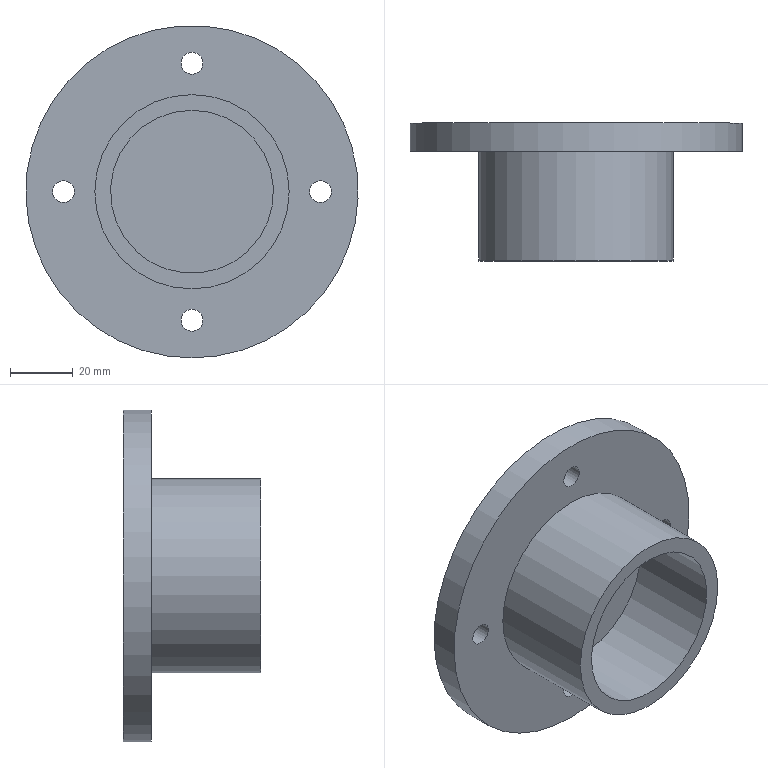Part | NX | features DATUM_CSYS 7, HOLE PACKAGE 6, SIMPLE HOLE 6, SKETCH 6, EXTRACT_DATUM_AXIS 4, EXTRACT_FACE 4, Instance Feature 3, EXTRUDE 2, OFFSET_REGION 1, Pattern Feature 1 | 1 solid | 13 faces | box 106 x 44 x 106 mm | volume 112067 mm3 | cylinder 8 | plane 5 | commonest cylinder face diameters 7 x4 52 x1 58 x1 62 x1 106 x1
STEP:
#1=CARTESIAN_POINT('',(0.,-9.,-53.));
#2=VERTEX_POINT('',#1);
#3=CARTESIAN_POINT('',(0.,-9.,0.));
#4=DIRECTION('',(0.,-1.,0.));
#5=DIRECTION('',(0.,0.,-1.));
#6=AXIS2_PLACEMENT_3D('',#3,#4,#5);
#7=CIRCLE('',#6,53.);
#8=EDGE_CURVE('',#2,#2,#7,.T.);
#9=ORIENTED_EDGE('',*,*,#8,.F.);
#10=EDGE_LOOP('',(#9));
#11=FACE_BOUND('',#10,.T.);
#12=CARTESIAN_POINT('',(0.,0.,-53.));
#13=VERTEX_POINT('',#12);
#14=CARTESIAN_POINT('',(0.,0.,0.));
#15=DIRECTION('',(0.,-1.,0.));
#16=DIRECTION('',(0.,0.,-1.));
#17=AXIS2_PLACEMENT_3D('',#14,#15,#16);
#18=CIRCLE('',#17,53.);
#19=EDGE_CURVE('',#13,#13,#18,.T.);
#20=ORIENTED_EDGE('',*,*,#19,.T.);
#21=EDGE_LOOP('',(#20));
#22=FACE_BOUND('',#21,.T.);
#23=CARTESIAN_POINT('',(0.,-9.,0.));
#24=DIRECTION('',(0.,1.,0.));
#25=DIRECTION('',(0.,0.,1.));
#26=AXIS2_PLACEMENT_3D('',#23,#24,#25);
#27=CYLINDRICAL_SURFACE('',#26,53.);
#28=ADVANCED_FACE('',(#11,#22),#27,.T.);
#29=CARTESIAN_POINT('',(0.,-9.,-44.5));
#30=VERTEX_POINT('',#29);
#31=CARTESIAN_POINT('',(0.,-9.,-41.));
#32=DIRECTION('',(0.,-1.,0.));
#33=DIRECTION('',(0.,0.,-1.));
#34=AXIS2_PLACEMENT_3D('',#31,#32,#33);
#35=CIRCLE('',#34,3.5);
#36=EDGE_CURVE('',#30,#30,#35,.T.);
#37=ORIENTED_EDGE('',*,*,#36,.F.);
#38=EDGE_LOOP('',(#37));
#39=FACE_BOUND('',#38,.T.);
#40=CARTESIAN_POINT('',(41.,-9.,-3.5));
#41=VERTEX_POINT('',#40);
#42=CARTESIAN_POINT('',(41.,-9.,0.));
#43=DIRECTION('',(0.,-1.,0.));
#44=DIRECTION('',(0.,0.,-1.));
#45=AXIS2_PLACEMENT_3D('',#42,#43,#44);
#46=CIRCLE('',#45,3.5);
#47=EDGE_CURVE('',#41,#41,#46,.T.);
#48=ORIENTED_EDGE('',*,*,#47,.F.);
#49=EDGE_LOOP('',(#48));
#50=FACE_BOUND('',#49,.T.);
#51=CARTESIAN_POINT('',(0.,-9.,37.5));
#52=VERTEX_POINT('',#51);
#53=CARTESIAN_POINT('',(0.,-9.,41.));
#54=DIRECTION('',(0.,-1.,0.));
#55=DIRECTION('',(0.,0.,-1.));
#56=AXIS2_PLACEMENT_3D('',#53,#54,#55);
#57=CIRCLE('',#56,3.5);
#58=EDGE_CURVE('',#52,#52,#57,.T.);
#59=ORIENTED_EDGE('',*,*,#58,.F.);
#60=EDGE_LOOP('',(#59));
#61=FACE_BOUND('',#60,.T.);
#62=CARTESIAN_POINT('',(-41.,-9.,-3.5));
#63=VERTEX_POINT('',#62);
#64=CARTESIAN_POINT('',(-41.,-9.,0.));
#65=DIRECTION('',(0.,-1.,0.));
#66=DIRECTION('',(0.,0.,-1.));
#67=AXIS2_PLACEMENT_3D('',#64,#65,#66);
#68=CIRCLE('',#67,3.5);
#69=EDGE_CURVE('',#63,#63,#68,.T.);
#70=ORIENTED_EDGE('',*,*,#69,.F.);
#71=EDGE_LOOP('',(#70));
#72=FACE_BOUND('',#71,.T.);
#73=CARTESIAN_POINT('',(31.,-9.,0.));
#74=VERTEX_POINT('',#73);
#75=CARTESIAN_POINT('',(0.,-9.,0.));
#76=DIRECTION('',(0.,-1.,0.));
#77=DIRECTION('',(1.,0.,0.));
#78=AXIS2_PLACEMENT_3D('',#75,#76,#77);
#79=CIRCLE('',#78,31.);
#80=EDGE_CURVE('',#74,#74,#79,.T.);
#81=ORIENTED_EDGE('',*,*,#80,.F.);
#82=EDGE_LOOP('',(#81));
#83=FACE_BOUND('',#82,.T.);
#84=ORIENTED_EDGE('',*,*,#8,.T.);
#85=EDGE_LOOP('',(#84));
#86=FACE_BOUND('',#85,.T.);
#87=CARTESIAN_POINT('',(0.,-9.,0.));
#88=DIRECTION('',(0.,-1.,0.));
#89=DIRECTION('',(0.,0.,-1.));
#90=AXIS2_PLACEMENT_3D('',#87,#88,#89);
#91=PLANE('',#90);
#92=ADVANCED_FACE('',(#39,#50,#61,#72,#83,#86),#91,.T.);
#93=CARTESIAN_POINT('',(0.,0.,-44.5));
#94=VERTEX_POINT('',#93);
#95=CARTESIAN_POINT('',(0.,0.,-41.));
#96=DIRECTION('',(0.,-1.,0.));
#97=DIRECTION('',(0.,0.,-1.));
#98=AXIS2_PLACEMENT_3D('',#95,#96,#97);
#99=CIRCLE('',#98,3.5);
#100=EDGE_CURVE('',#94,#94,#99,.T.);
#101=ORIENTED_EDGE('',*,*,#100,.T.);
#102=EDGE_LOOP('',(#101));
#103=FACE_BOUND('',#102,.T.);
#104=CARTESIAN_POINT('',(41.,0.,-3.5));
#105=VERTEX_POINT('',#104);
#106=CARTESIAN_POINT('',(41.,0.,0.));
#107=DIRECTION('',(0.,-1.,0.));
#108=DIRECTION('',(0.,0.,-1.));
#109=AXIS2_PLACEMENT_3D('',#106,#107,#108);
#110=CIRCLE('',#109,3.5);
#111=EDGE_CURVE('',#105,#105,#110,.T.);
#112=ORIENTED_EDGE('',*,*,#111,.T.);
#113=EDGE_LOOP('',(#112));
#114=FACE_BOUND('',#113,.T.);
#115=CARTESIAN_POINT('',(0.,0.,37.5));
#116=VERTEX_POINT('',#115);
#117=CARTESIAN_POINT('',(0.,0.,41.));
#118=DIRECTION('',(0.,-1.,0.));
#119=DIRECTION('',(0.,0.,-1.));
#120=AXIS2_PLACEMENT_3D('',#117,#118,#119);
#121=CIRCLE('',#120,3.5);
#122=EDGE_CURVE('',#116,#116,#121,.T.);
#123=ORIENTED_EDGE('',*,*,#122,.T.);
#124=EDGE_LOOP('',(#123));
#125=FACE_BOUND('',#124,.T.);
#126=CARTESIAN_POINT('',(-41.,0.,-3.5));
#127=VERTEX_POINT('',#126);
#128=CARTESIAN_POINT('',(-41.,0.,0.));
#129=DIRECTION('',(0.,-1.,0.));
#130=DIRECTION('',(0.,0.,-1.));
#131=AXIS2_PLACEMENT_3D('',#128,#129,#130);
#132=CIRCLE('',#131,3.5);
#133=EDGE_CURVE('',#127,#127,#132,.T.);
#134=ORIENTED_EDGE('',*,*,#133,.T.);
#135=EDGE_LOOP('',(#134));
#136=FACE_BOUND('',#135,.T.);
#137=CARTESIAN_POINT('',(0.,0.,-29.));
#138=VERTEX_POINT('',#137);
#139=CARTESIAN_POINT('',(0.,0.,0.));
#140=DIRECTION('',(0.,-1.,0.));
#141=DIRECTION('',(0.,0.,-1.));
#142=AXIS2_PLACEMENT_3D('',#139,#140,#141);
#143=CIRCLE('',#142,29.);
#144=EDGE_CURVE('',#138,#138,#143,.T.);
#145=ORIENTED_EDGE('',*,*,#144,.T.);
#146=EDGE_LOOP('',(#145));
#147=FACE_BOUND('',#146,.T.);
#148=ORIENTED_EDGE('',*,*,#19,.F.);
#149=EDGE_LOOP('',(#148));
#150=FACE_BOUND('',#149,.T.);
#151=CARTESIAN_POINT('',(0.,0.,0.));
#152=DIRECTION('',(0.,-1.,0.));
#153=DIRECTION('',(0.,0.,-1.));
#154=AXIS2_PLACEMENT_3D('',#151,#152,#153);
#155=PLANE('',#154);
#156=ADVANCED_FACE('',(#103,#114,#125,#136,#147,#150),#155,.F.);
#157=CARTESIAN_POINT('',(31.,-44.,0.));
#158=VERTEX_POINT('',#157);
#159=CARTESIAN_POINT('',(0.,-44.,0.));
#160=DIRECTION('',(0.,-1.,0.));
#161=DIRECTION('',(1.,0.,0.));
#162=AXIS2_PLACEMENT_3D('',#159,#160,#161);
#163=CIRCLE('',#162,31.);
#164=EDGE_CURVE('',#158,#158,#163,.T.);
#165=ORIENTED_EDGE('',*,*,#164,.F.);
#166=EDGE_LOOP('',(#165));
#167=FACE_BOUND('',#166,.T.);
#168=ORIENTED_EDGE('',*,*,#80,.T.);
#169=EDGE_LOOP('',(#168));
#170=FACE_BOUND('',#169,.T.);
#171=CARTESIAN_POINT('',(0.,-44.,0.));
#172=DIRECTION('',(0.,1.,0.));
#173=DIRECTION('',(0.,0.,1.));
#174=AXIS2_PLACEMENT_3D('',#171,#172,#173);
#175=CYLINDRICAL_SURFACE('',#174,31.);
#176=ADVANCED_FACE('',(#167,#170),#175,.T.);
#177=CARTESIAN_POINT('',(0.,-44.,26.));
#178=VERTEX_POINT('',#177);
#179=CARTESIAN_POINT('',(0.,-44.,0.));
#180=DIRECTION('',(0.,1.,0.));
#181=DIRECTION('',(0.,0.,1.));
#182=AXIS2_PLACEMENT_3D('',#179,#180,#181);
#183=CIRCLE('',#182,26.);
#184=EDGE_CURVE('',#178,#178,#183,.T.);
#185=ORIENTED_EDGE('',*,*,#184,.T.);
#186=EDGE_LOOP('',(#185));
#187=FACE_BOUND('',#186,.T.);
#188=ORIENTED_EDGE('',*,*,#164,.T.);
#189=EDGE_LOOP('',(#188));
#190=FACE_BOUND('',#189,.T.);
#191=CARTESIAN_POINT('',(0.,-44.,0.));
#192=DIRECTION('',(0.,-1.,0.));
#193=DIRECTION('',(0.,0.,-1.));
#194=AXIS2_PLACEMENT_3D('',#191,#192,#193);
#195=PLANE('',#194);
#196=ADVANCED_FACE('',(#187,#190),#195,.T.);
#197=CARTESIAN_POINT('',(0.,-14.,26.));
#198=VERTEX_POINT('',#197);
#199=CARTESIAN_POINT('',(0.,-14.,0.));
#200=DIRECTION('',(0.,1.,0.));
#201=DIRECTION('',(0.,0.,1.));
#202=AXIS2_PLACEMENT_3D('',#199,#200,#201);
#203=CIRCLE('',#202,26.);
#204=EDGE_CURVE('',#198,#198,#203,.F.);
#205=ORIENTED_EDGE('',*,*,#204,.T.);
#206=EDGE_LOOP('',(#205));
#207=FACE_BOUND('',#206,.T.);
#208=CARTESIAN_POINT('',(0.,-14.,0.));
#209=DIRECTION('',(0.,1.,0.));
#210=DIRECTION('',(0.,0.,1.));
#211=AXIS2_PLACEMENT_3D('',#208,#209,#210);
#212=PLANE('',#211);
#213=ADVANCED_FACE('',(#207),#212,.F.);
#214=ORIENTED_EDGE('',*,*,#204,.F.);
#215=EDGE_LOOP('',(#214));
#216=FACE_BOUND('',#215,.T.);
#217=ORIENTED_EDGE('',*,*,#184,.F.);
#218=EDGE_LOOP('',(#217));
#219=FACE_BOUND('',#218,.T.);
#220=CARTESIAN_POINT('',(0.,-44.,0.));
#221=DIRECTION('',(0.,1.,0.));
#222=DIRECTION('',(0.,0.,1.));
#223=AXIS2_PLACEMENT_3D('',#220,#221,#222);
#224=CYLINDRICAL_SURFACE('',#223,26.);
#225=ADVANCED_FACE('',(#216,#219),#224,.F.);
#226=CARTESIAN_POINT('',(0.,-3.,-29.));
#227=VERTEX_POINT('',#226);
#228=CARTESIAN_POINT('',(0.,-3.,0.));
#229=DIRECTION('',(0.,-1.,0.));
#230=DIRECTION('',(0.,0.,-1.));
#231=AXIS2_PLACEMENT_3D('',#228,#229,#230);
#232=CIRCLE('',#231,29.);
#233=EDGE_CURVE('',#227,#227,#232,.F.);
#234=ORIENTED_EDGE('',*,*,#233,.T.);
#235=EDGE_LOOP('',(#234));
#236=FACE_BOUND('',#235,.T.);
#237=CARTESIAN_POINT('',(0.,-3.,0.));
#238=DIRECTION('',(0.,-1.,0.));
#239=DIRECTION('',(0.,0.,-1.));
#240=AXIS2_PLACEMENT_3D('',#237,#238,#239);
#241=PLANE('',#240);
#242=ADVANCED_FACE('',(#236),#241,.F.);
#243=ORIENTED_EDGE('',*,*,#233,.F.);
#244=EDGE_LOOP('',(#243));
#245=FACE_BOUND('',#244,.T.);
#246=ORIENTED_EDGE('',*,*,#144,.F.);
#247=EDGE_LOOP('',(#246));
#248=FACE_BOUND('',#247,.T.);
#249=CARTESIAN_POINT('',(0.,0.,0.));
#250=DIRECTION('',(0.,-1.,0.));
#251=DIRECTION('',(0.,0.,-1.));
#252=AXIS2_PLACEMENT_3D('',#249,#250,#251);
#253=CYLINDRICAL_SURFACE('',#252,29.);
#254=ADVANCED_FACE('',(#245,#248),#253,.F.);
#255=ORIENTED_EDGE('',*,*,#69,.T.);
#256=EDGE_LOOP('',(#255));
#257=FACE_BOUND('',#256,.T.);
#258=ORIENTED_EDGE('',*,*,#133,.F.);
#259=EDGE_LOOP('',(#258));
#260=FACE_BOUND('',#259,.T.);
#261=CARTESIAN_POINT('',(-41.,0.,0.));
#262=DIRECTION('',(0.,-1.,0.));
#263=DIRECTION('',(0.,0.,-1.));
#264=AXIS2_PLACEMENT_3D('',#261,#262,#263);
#265=CYLINDRICAL_SURFACE('',#264,3.5);
#266=ADVANCED_FACE('',(#257,#260),#265,.F.);
#267=ORIENTED_EDGE('',*,*,#58,.T.);
#268=EDGE_LOOP('',(#267));
#269=FACE_BOUND('',#268,.T.);
#270=ORIENTED_EDGE('',*,*,#122,.F.);
#271=EDGE_LOOP('',(#270));
#272=FACE_BOUND('',#271,.T.);
#273=CARTESIAN_POINT('',(0.,0.,41.));
#274=DIRECTION('',(0.,-1.,0.));
#275=DIRECTION('',(0.,0.,-1.));
#276=AXIS2_PLACEMENT_3D('',#273,#274,#275);
#277=CYLINDRICAL_SURFACE('',#276,3.5);
#278=ADVANCED_FACE('',(#269,#272),#277,.F.);
#279=ORIENTED_EDGE('',*,*,#47,.T.);
#280=EDGE_LOOP('',(#279));
#281=FACE_BOUND('',#280,.T.);
#282=ORIENTED_EDGE('',*,*,#111,.F.);
#283=EDGE_LOOP('',(#282));
#284=FACE_BOUND('',#283,.T.);
#285=CARTESIAN_POINT('',(41.,0.,0.));
#286=DIRECTION('',(0.,-1.,0.));
#287=DIRECTION('',(0.,0.,-1.));
#288=AXIS2_PLACEMENT_3D('',#285,#286,#287);
#289=CYLINDRICAL_SURFACE('',#288,3.5);
#290=ADVANCED_FACE('',(#281,#284),#289,.F.);
#291=ORIENTED_EDGE('',*,*,#36,.T.);
#292=EDGE_LOOP('',(#291));
#293=FACE_BOUND('',#292,.T.);
#294=ORIENTED_EDGE('',*,*,#100,.F.);
#295=EDGE_LOOP('',(#294));
#296=FACE_BOUND('',#295,.T.);
#297=CARTESIAN_POINT('',(0.,0.,-41.));
#298=DIRECTION('',(0.,-1.,0.));
#299=DIRECTION('',(0.,0.,-1.));
#300=AXIS2_PLACEMENT_3D('',#297,#298,#299);
#301=CYLINDRICAL_SURFACE('',#300,3.5);
#302=ADVANCED_FACE('',(#293,#296),#301,.F.);
#303=CLOSED_SHELL('',(#28,#92,#156,#176,#196,#213,#225,#242,#254,#266,#278,#290,#302));
#304=MANIFOLD_SOLID_BREP('',#303);
#305=(LENGTH_UNIT()NAMED_UNIT(*)SI_UNIT(.MILLI.,.METRE.));
#306=UNCERTAINTY_MEASURE_WITH_UNIT(LENGTH_MEASURE(0.00001),#305,'','');
#307=(NAMED_UNIT(*)PLANE_ANGLE_UNIT()SI_UNIT($,.RADIAN.));
#308=(NAMED_UNIT(*)SI_UNIT($,.STERADIAN.)SOLID_ANGLE_UNIT());
#309=(GEOMETRIC_REPRESENTATION_CONTEXT(3)GLOBAL_UNCERTAINTY_ASSIGNED_CONTEXT((#306))GLOBAL_UNIT_ASSIGNED_CONTEXT((#305,#307,#308))REPRESENTATION_CONTEXT('',''));
#310=ADVANCED_BREP_SHAPE_REPRESENTATION('',(#304),#309);